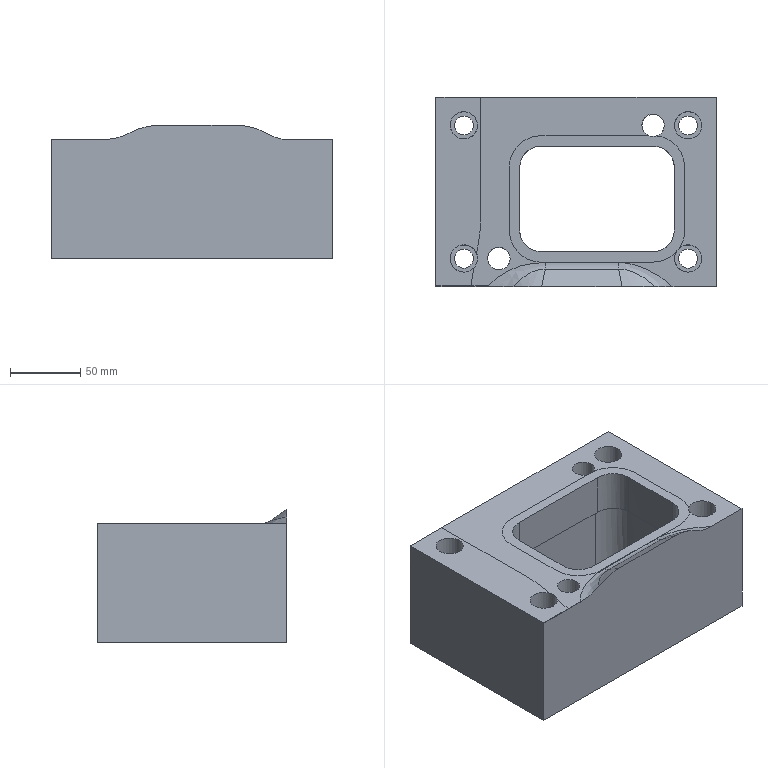Part | NX | features solid 2 | 1 solid | 42 faces | box 200 x 135 x 95.101 mm | volume 1451006 mm3 | spline 21 | plane 11 | cylinder 10 | commonest cylinder face diameters 13.5 x4 19.5 x4 16 x2